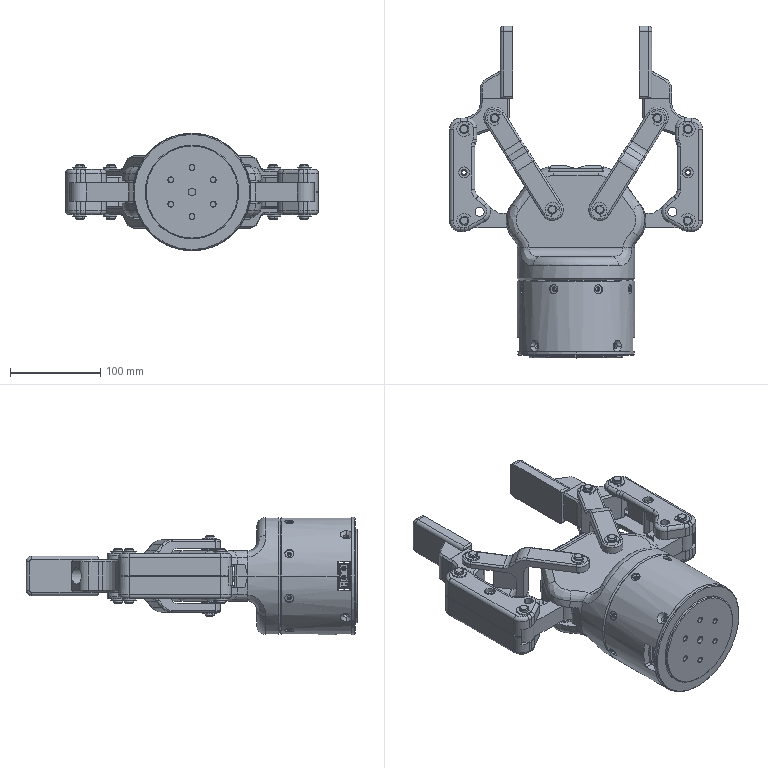Part | NX | features BREP 72 | 72 solids | 4489 faces | volume 2313606 mm3 | cylinder 2077 | plane 1557 | cone 413 | spline 350 | torus 92 | commonest cylinder face diameters 4 x341 5 x272 8 x179 10 x102 0.508 x96 2 x78